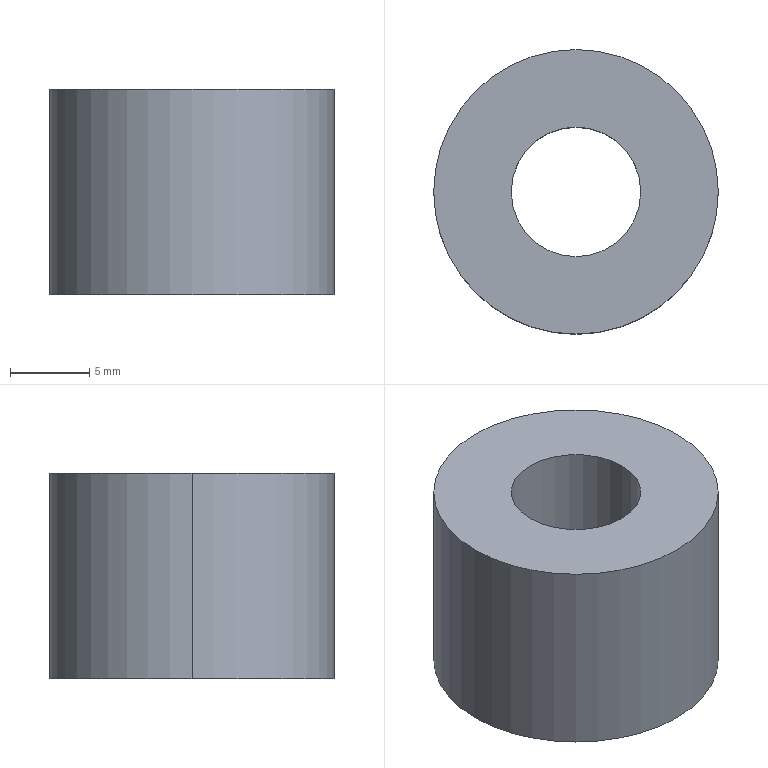Part | STEP file | A09 | 1 solid | 6 faces | box 18 x 18 x 13 mm | volume 2622 mm3 | cylinder 4 | plane 2 | commonest cylinder face diameters 8.2 x2 18 x2
STEP:
#1=CARTESIAN_POINT('',(0.,0.,0.));
#2=DIRECTION('',(0.,0.,1.));
#3=DIRECTION('',(1.,0.,0.));
#4=AXIS2_PLACEMENT_3D('',#1,#2,#3);
#5=CARTESIAN_POINT('',(-4.1,0.,13.));
#6=VERTEX_POINT('',#5);
#7=CARTESIAN_POINT('',(-4.1,0.,0.));
#8=VERTEX_POINT('',#7);
#9=CARTESIAN_POINT('',(-4.1,0.,13.));
#10=DIRECTION('',(0.,0.,-1.));
#11=VECTOR('',#10,1.);
#12=LINE('',#9,#11);
#13=CARTESIAN_POINT('',(0.,0.,13.));
#14=DIRECTION('',(0.,0.,-1.));
#15=DIRECTION('',(-1.,0.,0.));
#16=AXIS2_PLACEMENT_3D('',#13,#14,#15);
#17=CYLINDRICAL_SURFACE('',#16,4.1);
#18=CARTESIAN_POINT('',(6.283,0.));
#19=DIRECTION('',(0.,1.));
#20=VECTOR('',#19,1.);
#21=LINE('',#18,#20);
#22=(GEOMETRIC_REPRESENTATION_CONTEXT(2)PARAMETRIC_REPRESENTATION_CONTEXT()REPRESENTATION_CONTEXT('',''));
#23=DEFINITIONAL_REPRESENTATION('',(#21),#22);
#24=PCURVE('',#17,#23);
#25=CARTESIAN_POINT('',(0.,0.,13.));
#26=DIRECTION('',(0.,0.,-1.));
#27=DIRECTION('',(-1.,0.,0.));
#28=AXIS2_PLACEMENT_3D('',#25,#26,#27);
#29=CYLINDRICAL_SURFACE('',#28,4.1);
#30=CARTESIAN_POINT('',(0.,0.));
#31=DIRECTION('',(0.,1.));
#32=VECTOR('',#31,1.);
#33=LINE('',#30,#32);
#34=(GEOMETRIC_REPRESENTATION_CONTEXT(2)PARAMETRIC_REPRESENTATION_CONTEXT()REPRESENTATION_CONTEXT('',''));
#35=DEFINITIONAL_REPRESENTATION('',(#33),#34);
#36=PCURVE('',#29,#35);
#37=SURFACE_CURVE('',#12,(#24,#36),.PCURVE_S1.);
#38=EDGE_CURVE('',#6,#8,#37,.T.);
#39=ORIENTED_EDGE('',*,*,#38,.T.);
#40=CARTESIAN_POINT('',(4.1,0.,0.));
#41=VERTEX_POINT('',#40);
#42=CARTESIAN_POINT('',(0.,0.,0.));
#43=DIRECTION('',(0.,0.,1.));
#44=DIRECTION('',(1.,0.,0.));
#45=AXIS2_PLACEMENT_3D('',#42,#43,#44);
#46=CIRCLE('',#45,4.1);
#47=CARTESIAN_POINT('',(9.425,13.));
#48=DIRECTION('',(-1.,0.));
#49=VECTOR('',#48,1.);
#50=LINE('',#47,#49);
#51=(GEOMETRIC_REPRESENTATION_CONTEXT(2)PARAMETRIC_REPRESENTATION_CONTEXT()REPRESENTATION_CONTEXT('',''));
#52=DEFINITIONAL_REPRESENTATION('',(#50),#51);
#53=PCURVE('',#17,#52);
#54=CARTESIAN_POINT('',(0.,0.,0.));
#55=DIRECTION('',(0.,0.,1.));
#56=DIRECTION('',(1.,0.,0.));
#57=AXIS2_PLACEMENT_3D('',#54,#55,#56);
#58=PLANE('',#57);
#59=CARTESIAN_POINT('',(0.,0.));
#60=DIRECTION('',(1.,0.));
#61=AXIS2_PLACEMENT_2D('',#59,#60);
#62=CIRCLE('',#61,4.1);
#63=(GEOMETRIC_REPRESENTATION_CONTEXT(2)PARAMETRIC_REPRESENTATION_CONTEXT()REPRESENTATION_CONTEXT('',''));
#64=DEFINITIONAL_REPRESENTATION('',(#62),#63);
#65=PCURVE('',#58,#64);
#66=SURFACE_CURVE('',#46,(#53,#65),.PCURVE_S1.);
#67=EDGE_CURVE('',#8,#41,#66,.T.);
#68=ORIENTED_EDGE('',*,*,#67,.T.);
#69=CARTESIAN_POINT('',(4.1,0.,13.));
#70=VERTEX_POINT('',#69);
#71=CARTESIAN_POINT('',(4.1,0.,13.));
#72=DIRECTION('',(0.,0.,-1.));
#73=VECTOR('',#72,1.);
#74=LINE('',#71,#73);
#75=CARTESIAN_POINT('',(3.142,0.));
#76=DIRECTION('',(0.,1.));
#77=VECTOR('',#76,1.);
#78=LINE('',#75,#77);
#79=(GEOMETRIC_REPRESENTATION_CONTEXT(2)PARAMETRIC_REPRESENTATION_CONTEXT()REPRESENTATION_CONTEXT('',''));
#80=DEFINITIONAL_REPRESENTATION('',(#78),#79);
#81=PCURVE('',#17,#80);
#82=CARTESIAN_POINT('',(3.142,0.));
#83=DIRECTION('',(0.,1.));
#84=VECTOR('',#83,1.);
#85=LINE('',#82,#84);
#86=(GEOMETRIC_REPRESENTATION_CONTEXT(2)PARAMETRIC_REPRESENTATION_CONTEXT()REPRESENTATION_CONTEXT('',''));
#87=DEFINITIONAL_REPRESENTATION('',(#85),#86);
#88=PCURVE('',#29,#87);
#89=SURFACE_CURVE('',#74,(#81,#88),.PCURVE_S1.);
#90=EDGE_CURVE('',#70,#41,#89,.T.);
#91=ORIENTED_EDGE('',*,*,#90,.F.);
#92=CARTESIAN_POINT('',(0.,0.,13.));
#93=DIRECTION('',(0.,0.,1.));
#94=DIRECTION('',(1.,0.,0.));
#95=AXIS2_PLACEMENT_3D('',#92,#93,#94);
#96=CIRCLE('',#95,4.1);
#97=CARTESIAN_POINT('',(9.425,0.));
#98=DIRECTION('',(-1.,0.));
#99=VECTOR('',#98,1.);
#100=LINE('',#97,#99);
#101=(GEOMETRIC_REPRESENTATION_CONTEXT(2)PARAMETRIC_REPRESENTATION_CONTEXT()REPRESENTATION_CONTEXT('',''));
#102=DEFINITIONAL_REPRESENTATION('',(#100),#101);
#103=PCURVE('',#17,#102);
#104=CARTESIAN_POINT('',(0.,0.,13.));
#105=DIRECTION('',(0.,0.,1.));
#106=DIRECTION('',(1.,0.,0.));
#107=AXIS2_PLACEMENT_3D('',#104,#105,#106);
#108=PLANE('',#107);
#109=CARTESIAN_POINT('',(0.,0.));
#110=DIRECTION('',(1.,0.));
#111=AXIS2_PLACEMENT_2D('',#109,#110);
#112=CIRCLE('',#111,4.1);
#113=(GEOMETRIC_REPRESENTATION_CONTEXT(2)PARAMETRIC_REPRESENTATION_CONTEXT()REPRESENTATION_CONTEXT('',''));
#114=DEFINITIONAL_REPRESENTATION('',(#112),#113);
#115=PCURVE('',#108,#114);
#116=SURFACE_CURVE('',#96,(#103,#115),.PCURVE_S1.);
#117=EDGE_CURVE('',#6,#70,#116,.T.);
#118=ORIENTED_EDGE('',*,*,#117,.F.);
#119=EDGE_LOOP('',(#39,#68,#91,#118));
#120=FACE_BOUND('',#119,.F.);
#121=ADVANCED_FACE('',(#120),#17,.F.);
#122=CARTESIAN_POINT('',(9.,0.,13.));
#123=VERTEX_POINT('',#122);
#124=CARTESIAN_POINT('',(-9.,0.,13.));
#125=VERTEX_POINT('',#124);
#126=CARTESIAN_POINT('',(0.,0.,13.));
#127=DIRECTION('',(0.,0.,1.));
#128=DIRECTION('',(1.,0.,0.));
#129=AXIS2_PLACEMENT_3D('',#126,#127,#128);
#130=CIRCLE('',#129,9.);
#131=CARTESIAN_POINT('',(0.,0.,13.));
#132=DIRECTION('',(0.,0.,-1.));
#133=DIRECTION('',(-1.,0.,0.));
#134=AXIS2_PLACEMENT_3D('',#131,#132,#133);
#135=CYLINDRICAL_SURFACE('',#134,9.);
#136=CARTESIAN_POINT('',(3.142,0.));
#137=DIRECTION('',(-1.,0.));
#138=VECTOR('',#137,1.);
#139=LINE('',#136,#138);
#140=(GEOMETRIC_REPRESENTATION_CONTEXT(2)PARAMETRIC_REPRESENTATION_CONTEXT()REPRESENTATION_CONTEXT('',''));
#141=DEFINITIONAL_REPRESENTATION('',(#139),#140);
#142=PCURVE('',#135,#141);
#143=CARTESIAN_POINT('',(0.,0.));
#144=DIRECTION('',(1.,0.));
#145=AXIS2_PLACEMENT_2D('',#143,#144);
#146=CIRCLE('',#145,9.);
#147=(GEOMETRIC_REPRESENTATION_CONTEXT(2)PARAMETRIC_REPRESENTATION_CONTEXT()REPRESENTATION_CONTEXT('',''));
#148=DEFINITIONAL_REPRESENTATION('',(#146),#147);
#149=PCURVE('',#108,#148);
#150=SURFACE_CURVE('',#130,(#142,#149),.PCURVE_S1.);
#151=EDGE_CURVE('',#123,#125,#150,.T.);
#152=ORIENTED_EDGE('',*,*,#151,.F.);
#153=CARTESIAN_POINT('',(9.,0.,0.));
#154=VERTEX_POINT('',#153);
#155=CARTESIAN_POINT('',(9.,0.,13.));
#156=DIRECTION('',(0.,0.,-1.));
#157=VECTOR('',#156,1.);
#158=LINE('',#155,#157);
#159=CARTESIAN_POINT('',(3.142,0.));
#160=DIRECTION('',(0.,1.));
#161=VECTOR('',#160,1.);
#162=LINE('',#159,#161);
#163=(GEOMETRIC_REPRESENTATION_CONTEXT(2)PARAMETRIC_REPRESENTATION_CONTEXT()REPRESENTATION_CONTEXT('',''));
#164=DEFINITIONAL_REPRESENTATION('',(#162),#163);
#165=PCURVE('',#135,#164);
#166=CARTESIAN_POINT('',(0.,0.,13.));
#167=DIRECTION('',(0.,0.,-1.));
#168=DIRECTION('',(-1.,0.,0.));
#169=AXIS2_PLACEMENT_3D('',#166,#167,#168);
#170=CYLINDRICAL_SURFACE('',#169,9.);
#171=CARTESIAN_POINT('',(3.142,0.));
#172=DIRECTION('',(0.,1.));
#173=VECTOR('',#172,1.);
#174=LINE('',#171,#173);
#175=(GEOMETRIC_REPRESENTATION_CONTEXT(2)PARAMETRIC_REPRESENTATION_CONTEXT()REPRESENTATION_CONTEXT('',''));
#176=DEFINITIONAL_REPRESENTATION('',(#174),#175);
#177=PCURVE('',#170,#176);
#178=SURFACE_CURVE('',#158,(#165,#177),.PCURVE_S1.);
#179=EDGE_CURVE('',#123,#154,#178,.T.);
#180=ORIENTED_EDGE('',*,*,#179,.T.);
#181=CARTESIAN_POINT('',(-9.,0.,0.));
#182=VERTEX_POINT('',#181);
#183=CARTESIAN_POINT('',(0.,0.,0.));
#184=DIRECTION('',(0.,0.,1.));
#185=DIRECTION('',(1.,0.,0.));
#186=AXIS2_PLACEMENT_3D('',#183,#184,#185);
#187=CIRCLE('',#186,9.);
#188=CARTESIAN_POINT('',(3.142,13.));
#189=DIRECTION('',(-1.,0.));
#190=VECTOR('',#189,1.);
#191=LINE('',#188,#190);
#192=(GEOMETRIC_REPRESENTATION_CONTEXT(2)PARAMETRIC_REPRESENTATION_CONTEXT()REPRESENTATION_CONTEXT('',''));
#193=DEFINITIONAL_REPRESENTATION('',(#191),#192);
#194=PCURVE('',#135,#193);
#195=CARTESIAN_POINT('',(0.,0.));
#196=DIRECTION('',(1.,0.));
#197=AXIS2_PLACEMENT_2D('',#195,#196);
#198=CIRCLE('',#197,9.);
#199=(GEOMETRIC_REPRESENTATION_CONTEXT(2)PARAMETRIC_REPRESENTATION_CONTEXT()REPRESENTATION_CONTEXT('',''));
#200=DEFINITIONAL_REPRESENTATION('',(#198),#199);
#201=PCURVE('',#58,#200);
#202=SURFACE_CURVE('',#187,(#194,#201),.PCURVE_S1.);
#203=EDGE_CURVE('',#154,#182,#202,.T.);
#204=ORIENTED_EDGE('',*,*,#203,.T.);
#205=CARTESIAN_POINT('',(-9.,0.,13.));
#206=DIRECTION('',(0.,0.,-1.));
#207=VECTOR('',#206,1.);
#208=LINE('',#205,#207);
#209=CARTESIAN_POINT('',(0.,0.));
#210=DIRECTION('',(0.,1.));
#211=VECTOR('',#210,1.);
#212=LINE('',#209,#211);
#213=(GEOMETRIC_REPRESENTATION_CONTEXT(2)PARAMETRIC_REPRESENTATION_CONTEXT()REPRESENTATION_CONTEXT('',''));
#214=DEFINITIONAL_REPRESENTATION('',(#212),#213);
#215=PCURVE('',#135,#214);
#216=CARTESIAN_POINT('',(6.283,0.));
#217=DIRECTION('',(0.,1.));
#218=VECTOR('',#217,1.);
#219=LINE('',#216,#218);
#220=(GEOMETRIC_REPRESENTATION_CONTEXT(2)PARAMETRIC_REPRESENTATION_CONTEXT()REPRESENTATION_CONTEXT('',''));
#221=DEFINITIONAL_REPRESENTATION('',(#219),#220);
#222=PCURVE('',#170,#221);
#223=SURFACE_CURVE('',#208,(#215,#222),.PCURVE_S1.);
#224=EDGE_CURVE('',#125,#182,#223,.T.);
#225=ORIENTED_EDGE('',*,*,#224,.F.);
#226=EDGE_LOOP('',(#152,#180,#204,#225));
#227=FACE_BOUND('',#226,.T.);
#228=ADVANCED_FACE('',(#227),#135,.T.);
#229=CARTESIAN_POINT('',(0.,0.,13.));
#230=DIRECTION('',(0.,0.,1.));
#231=DIRECTION('',(1.,0.,0.));
#232=AXIS2_PLACEMENT_3D('',#229,#230,#231);
#233=CIRCLE('',#232,9.);
#234=CARTESIAN_POINT('',(0.,0.));
#235=DIRECTION('',(1.,0.));
#236=AXIS2_PLACEMENT_2D('',#234,#235);
#237=CIRCLE('',#236,9.);
#238=(GEOMETRIC_REPRESENTATION_CONTEXT(2)PARAMETRIC_REPRESENTATION_CONTEXT()REPRESENTATION_CONTEXT('',''));
#239=DEFINITIONAL_REPRESENTATION('',(#237),#238);
#240=PCURVE('',#108,#239);
#241=CARTESIAN_POINT('',(9.425,0.));
#242=DIRECTION('',(-1.,0.));
#243=VECTOR('',#242,1.);
#244=LINE('',#241,#243);
#245=(GEOMETRIC_REPRESENTATION_CONTEXT(2)PARAMETRIC_REPRESENTATION_CONTEXT()REPRESENTATION_CONTEXT('',''));
#246=DEFINITIONAL_REPRESENTATION('',(#244),#245);
#247=PCURVE('',#170,#246);
#248=SURFACE_CURVE('',#233,(#240,#247),.PCURVE_S1.);
#249=EDGE_CURVE('',#125,#123,#248,.T.);
#250=ORIENTED_EDGE('',*,*,#249,.T.);
#251=ORIENTED_EDGE('',*,*,#151,.T.);
#252=EDGE_LOOP('',(#250,#251));
#253=FACE_BOUND('',#252,.T.);
#254=ORIENTED_EDGE('',*,*,#117,.F.);
#255=CARTESIAN_POINT('',(0.,0.,13.));
#256=DIRECTION('',(0.,0.,1.));
#257=DIRECTION('',(1.,0.,0.));
#258=AXIS2_PLACEMENT_3D('',#255,#256,#257);
#259=CIRCLE('',#258,4.1);
#260=CARTESIAN_POINT('',(0.,0.));
#261=DIRECTION('',(1.,0.));
#262=AXIS2_PLACEMENT_2D('',#260,#261);
#263=CIRCLE('',#262,4.1);
#264=(GEOMETRIC_REPRESENTATION_CONTEXT(2)PARAMETRIC_REPRESENTATION_CONTEXT()REPRESENTATION_CONTEXT('',''));
#265=DEFINITIONAL_REPRESENTATION('',(#263),#264);
#266=PCURVE('',#108,#265);
#267=CARTESIAN_POINT('',(3.142,0.));
#268=DIRECTION('',(-1.,0.));
#269=VECTOR('',#268,1.);
#270=LINE('',#267,#269);
#271=(GEOMETRIC_REPRESENTATION_CONTEXT(2)PARAMETRIC_REPRESENTATION_CONTEXT()REPRESENTATION_CONTEXT('',''));
#272=DEFINITIONAL_REPRESENTATION('',(#270),#271);
#273=PCURVE('',#29,#272);
#274=SURFACE_CURVE('',#259,(#266,#273),.PCURVE_S1.);
#275=EDGE_CURVE('',#70,#6,#274,.T.);
#276=ORIENTED_EDGE('',*,*,#275,.F.);
#277=EDGE_LOOP('',(#254,#276));
#278=FACE_BOUND('',#277,.T.);
#279=ADVANCED_FACE('',(#253,#278),#108,.T.);
#280=CARTESIAN_POINT('',(0.,0.,0.));
#281=DIRECTION('',(0.,0.,1.));
#282=DIRECTION('',(1.,0.,0.));
#283=AXIS2_PLACEMENT_3D('',#280,#281,#282);
#284=CIRCLE('',#283,9.);
#285=CARTESIAN_POINT('',(0.,0.));
#286=DIRECTION('',(1.,0.));
#287=AXIS2_PLACEMENT_2D('',#285,#286);
#288=CIRCLE('',#287,9.);
#289=(GEOMETRIC_REPRESENTATION_CONTEXT(2)PARAMETRIC_REPRESENTATION_CONTEXT()REPRESENTATION_CONTEXT('',''));
#290=DEFINITIONAL_REPRESENTATION('',(#288),#289);
#291=PCURVE('',#58,#290);
#292=CARTESIAN_POINT('',(9.425,13.));
#293=DIRECTION('',(-1.,0.));
#294=VECTOR('',#293,1.);
#295=LINE('',#292,#294);
#296=(GEOMETRIC_REPRESENTATION_CONTEXT(2)PARAMETRIC_REPRESENTATION_CONTEXT()REPRESENTATION_CONTEXT('',''));
#297=DEFINITIONAL_REPRESENTATION('',(#295),#296);
#298=PCURVE('',#170,#297);
#299=SURFACE_CURVE('',#284,(#291,#298),.PCURVE_S1.);
#300=EDGE_CURVE('',#182,#154,#299,.T.);
#301=ORIENTED_EDGE('',*,*,#300,.F.);
#302=ORIENTED_EDGE('',*,*,#203,.F.);
#303=EDGE_LOOP('',(#301,#302));
#304=FACE_BOUND('',#303,.T.);
#305=ORIENTED_EDGE('',*,*,#67,.T.);
#306=CARTESIAN_POINT('',(0.,0.,0.));
#307=DIRECTION('',(0.,0.,1.));
#308=DIRECTION('',(1.,0.,0.));
#309=AXIS2_PLACEMENT_3D('',#306,#307,#308);
#310=CIRCLE('',#309,4.1);
#311=CARTESIAN_POINT('',(0.,0.));
#312=DIRECTION('',(1.,0.));
#313=AXIS2_PLACEMENT_2D('',#311,#312);
#314=CIRCLE('',#313,4.1);
#315=(GEOMETRIC_REPRESENTATION_CONTEXT(2)PARAMETRIC_REPRESENTATION_CONTEXT()REPRESENTATION_CONTEXT('',''));
#316=DEFINITIONAL_REPRESENTATION('',(#314),#315);
#317=PCURVE('',#58,#316);
#318=CARTESIAN_POINT('',(3.142,13.));
#319=DIRECTION('',(-1.,0.));
#320=VECTOR('',#319,1.);
#321=LINE('',#318,#320);
#322=(GEOMETRIC_REPRESENTATION_CONTEXT(2)PARAMETRIC_REPRESENTATION_CONTEXT()REPRESENTATION_CONTEXT('',''));
#323=DEFINITIONAL_REPRESENTATION('',(#321),#322);
#324=PCURVE('',#29,#323);
#325=SURFACE_CURVE('',#310,(#317,#324),.PCURVE_S1.);
#326=EDGE_CURVE('',#41,#8,#325,.T.);
#327=ORIENTED_EDGE('',*,*,#326,.T.);
#328=EDGE_LOOP('',(#305,#327));
#329=FACE_BOUND('',#328,.T.);
#330=ADVANCED_FACE('',(#304,#329),#58,.F.);
#331=ORIENTED_EDGE('',*,*,#179,.F.);
#332=ORIENTED_EDGE('',*,*,#249,.F.);
#333=ORIENTED_EDGE('',*,*,#224,.T.);
#334=ORIENTED_EDGE('',*,*,#300,.T.);
#335=EDGE_LOOP('',(#331,#332,#333,#334));
#336=FACE_BOUND('',#335,.T.);
#337=ADVANCED_FACE('',(#336),#170,.T.);
#338=ORIENTED_EDGE('',*,*,#326,.T.);
#339=ORIENTED_EDGE('',*,*,#38,.F.);
#340=ORIENTED_EDGE('',*,*,#275,.F.);
#341=ORIENTED_EDGE('',*,*,#90,.T.);
#342=EDGE_LOOP('',(#338,#339,#340,#341));
#343=FACE_BOUND('',#342,.F.);
#344=ADVANCED_FACE('',(#343),#29,.F.);
#345=CLOSED_SHELL('',(#121,#228,#279,#330,#337,#344));
#346=MANIFOLD_SOLID_BREP('',#345);
#347=(LENGTH_UNIT()NAMED_UNIT(*)SI_UNIT(.MILLI.,.METRE.));
#348=UNCERTAINTY_MEASURE_WITH_UNIT(LENGTH_MEASURE(0.0000001),#347,'','');
#349=(NAMED_UNIT(*)PLANE_ANGLE_UNIT()SI_UNIT($,.RADIAN.));
#350=(NAMED_UNIT(*)SI_UNIT($,.STERADIAN.)SOLID_ANGLE_UNIT());
#351=(GEOMETRIC_REPRESENTATION_CONTEXT(3)GLOBAL_UNCERTAINTY_ASSIGNED_CONTEXT((#348))GLOBAL_UNIT_ASSIGNED_CONTEXT((#347,#349,#350))REPRESENTATION_CONTEXT('',''));
#352=ADVANCED_BREP_SHAPE_REPRESENTATION('',(#4,#346),#351);